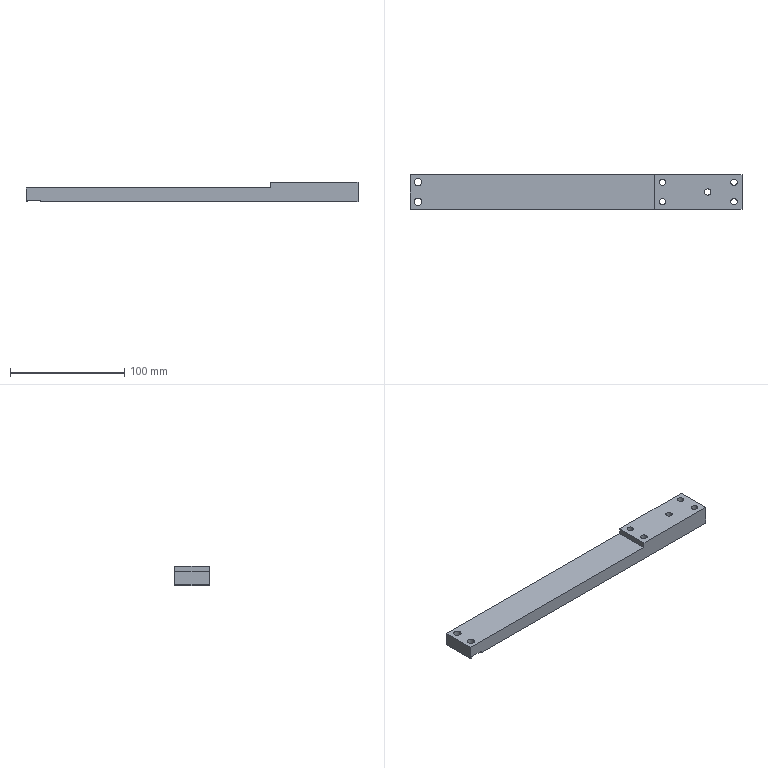Part | NX | features BREP 1 | 1 solid | 45 faces | box 290 x 30 x 17 mm | volume 111085 mm3 | cylinder 26 | plane 17 | cone 2 | commonest cylinder face diameters 5.5 x10 10 x10 6.5 x4 3.3 x2
STEP:
#1=CARTESIAN_POINT('',(-455.312,44.77,5.));
#2=VERTEX_POINT('',#1);
#3=CARTESIAN_POINT('',(-465.312,44.77,5.));
#4=VERTEX_POINT('',#3);
#5=CARTESIAN_POINT('',(-460.312,44.77,5.));
#6=DIRECTION('',(0.,0.,-1.));
#7=DIRECTION('',(-1.,0.,0.));
#8=AXIS2_PLACEMENT_3D('',#5,#6,#7);
#9=CIRCLE('',#8,5.);
#10=EDGE_CURVE('',#2,#4,#9,.T.);
#11=ORIENTED_EDGE('',*,*,#10,.F.);
#12=CARTESIAN_POINT('',(-455.312,44.77,0.));
#13=VERTEX_POINT('',#12);
#14=CARTESIAN_POINT('',(-455.312,44.77,0.));
#15=DIRECTION('',(0.,0.,-1.));
#16=VECTOR('',#15,1000.);
#17=LINE('',#14,#16);
#18=EDGE_CURVE('',#2,#13,#17,.T.);
#19=ORIENTED_EDGE('',*,*,#18,.T.);
#20=CARTESIAN_POINT('',(-465.312,44.77,0.));
#21=VERTEX_POINT('',#20);
#22=CARTESIAN_POINT('',(-460.312,44.77,0.));
#23=DIRECTION('',(0.,0.,-1.));
#24=DIRECTION('',(-1.,0.,0.));
#25=AXIS2_PLACEMENT_3D('',#22,#23,#24);
#26=CIRCLE('',#25,5.);
#27=EDGE_CURVE('',#13,#21,#26,.T.);
#28=ORIENTED_EDGE('',*,*,#27,.T.);
#29=CARTESIAN_POINT('',(-465.312,44.77,0.));
#30=DIRECTION('',(0.,0.,-1.));
#31=VECTOR('',#30,1000.);
#32=LINE('',#29,#31);
#33=EDGE_CURVE('',#4,#21,#32,.T.);
#34=ORIENTED_EDGE('',*,*,#33,.F.);
#35=EDGE_LOOP('',(#11,#19,#28,#34));
#36=FACE_BOUND('',#35,.T.);
#37=CARTESIAN_POINT('',(-460.312,44.77,0.));
#38=DIRECTION('',(0.,0.,-1.));
#39=DIRECTION('',(-1.,0.,0.));
#40=AXIS2_PLACEMENT_3D('',#37,#38,#39);
#41=CYLINDRICAL_SURFACE('',#40,5.);
#42=ADVANCED_FACE('',(#36),#41,.F.);
#43=CARTESIAN_POINT('',(-463.062,44.77,17.));
#44=VERTEX_POINT('',#43);
#45=CARTESIAN_POINT('',(-457.562,44.77,17.));
#46=VERTEX_POINT('',#45);
#47=CARTESIAN_POINT('',(-460.312,44.77,17.));
#48=DIRECTION('',(0.,0.,1.));
#49=DIRECTION('',(1.,0.,0.));
#50=AXIS2_PLACEMENT_3D('',#47,#48,#49);
#51=CIRCLE('',#50,2.75);
#52=EDGE_CURVE('',#44,#46,#51,.T.);
#53=ORIENTED_EDGE('',*,*,#52,.T.);
#54=CARTESIAN_POINT('',(-457.562,44.77,5.));
#55=VERTEX_POINT('',#54);
#56=CARTESIAN_POINT('',(-457.562,44.77,0.));
#57=DIRECTION('',(0.,0.,-1.));
#58=VECTOR('',#57,1000.);
#59=LINE('',#56,#58);
#60=EDGE_CURVE('',#46,#55,#59,.T.);
#61=ORIENTED_EDGE('',*,*,#60,.T.);
#62=CARTESIAN_POINT('',(-463.062,44.77,5.));
#63=VERTEX_POINT('',#62);
#64=CARTESIAN_POINT('',(-460.312,44.77,5.));
#65=DIRECTION('',(0.,0.,-1.));
#66=DIRECTION('',(-1.,0.,0.));
#67=AXIS2_PLACEMENT_3D('',#64,#65,#66);
#68=CIRCLE('',#67,2.75);
#69=EDGE_CURVE('',#55,#63,#68,.T.);
#70=ORIENTED_EDGE('',*,*,#69,.T.);
#71=CARTESIAN_POINT('',(-463.062,44.77,0.));
#72=DIRECTION('',(0.,0.,-1.));
#73=VECTOR('',#72,1000.);
#74=LINE('',#71,#73);
#75=EDGE_CURVE('',#44,#63,#74,.T.);
#76=ORIENTED_EDGE('',*,*,#75,.F.);
#77=EDGE_LOOP('',(#53,#61,#70,#76));
#78=FACE_BOUND('',#77,.T.);
#79=CARTESIAN_POINT('',(-460.312,44.77,0.));
#80=DIRECTION('',(0.,0.,-1.));
#81=DIRECTION('',(-1.,0.,0.));
#82=AXIS2_PLACEMENT_3D('',#79,#80,#81);
#83=CYLINDRICAL_SURFACE('',#82,2.75);
#84=ADVANCED_FACE('',(#78),#83,.F.);
#85=CARTESIAN_POINT('',(-455.312,27.77,5.));
#86=VERTEX_POINT('',#85);
#87=CARTESIAN_POINT('',(-465.312,27.77,5.));
#88=VERTEX_POINT('',#87);
#89=CARTESIAN_POINT('',(-460.312,27.77,5.));
#90=DIRECTION('',(0.,0.,-1.));
#91=DIRECTION('',(-1.,0.,0.));
#92=AXIS2_PLACEMENT_3D('',#89,#90,#91);
#93=CIRCLE('',#92,5.);
#94=EDGE_CURVE('',#86,#88,#93,.T.);
#95=ORIENTED_EDGE('',*,*,#94,.F.);
#96=CARTESIAN_POINT('',(-455.312,27.77,0.));
#97=VERTEX_POINT('',#96);
#98=CARTESIAN_POINT('',(-455.312,27.77,0.));
#99=DIRECTION('',(0.,0.,-1.));
#100=VECTOR('',#99,1000.);
#101=LINE('',#98,#100);
#102=EDGE_CURVE('',#86,#97,#101,.T.);
#103=ORIENTED_EDGE('',*,*,#102,.T.);
#104=CARTESIAN_POINT('',(-465.312,27.77,0.));
#105=VERTEX_POINT('',#104);
#106=CARTESIAN_POINT('',(-460.312,27.77,0.));
#107=DIRECTION('',(0.,0.,-1.));
#108=DIRECTION('',(-1.,0.,0.));
#109=AXIS2_PLACEMENT_3D('',#106,#107,#108);
#110=CIRCLE('',#109,5.);
#111=EDGE_CURVE('',#97,#105,#110,.T.);
#112=ORIENTED_EDGE('',*,*,#111,.T.);
#113=CARTESIAN_POINT('',(-465.312,27.77,0.));
#114=DIRECTION('',(0.,0.,-1.));
#115=VECTOR('',#114,1000.);
#116=LINE('',#113,#115);
#117=EDGE_CURVE('',#88,#105,#116,.T.);
#118=ORIENTED_EDGE('',*,*,#117,.F.);
#119=EDGE_LOOP('',(#95,#103,#112,#118));
#120=FACE_BOUND('',#119,.T.);
#121=CARTESIAN_POINT('',(-460.312,27.77,0.));
#122=DIRECTION('',(0.,0.,-1.));
#123=DIRECTION('',(-1.,0.,0.));
#124=AXIS2_PLACEMENT_3D('',#121,#122,#123);
#125=CYLINDRICAL_SURFACE('',#124,5.);
#126=ADVANCED_FACE('',(#120),#125,.F.);
#127=CARTESIAN_POINT('',(-463.062,27.77,17.));
#128=VERTEX_POINT('',#127);
#129=CARTESIAN_POINT('',(-457.562,27.77,17.));
#130=VERTEX_POINT('',#129);
#131=CARTESIAN_POINT('',(-460.312,27.77,17.));
#132=DIRECTION('',(0.,0.,1.));
#133=DIRECTION('',(1.,0.,0.));
#134=AXIS2_PLACEMENT_3D('',#131,#132,#133);
#135=CIRCLE('',#134,2.75);
#136=EDGE_CURVE('',#128,#130,#135,.T.);
#137=ORIENTED_EDGE('',*,*,#136,.T.);
#138=CARTESIAN_POINT('',(-457.562,27.77,5.));
#139=VERTEX_POINT('',#138);
#140=CARTESIAN_POINT('',(-457.562,27.77,0.));
#141=DIRECTION('',(0.,0.,-1.));
#142=VECTOR('',#141,1000.);
#143=LINE('',#140,#142);
#144=EDGE_CURVE('',#130,#139,#143,.T.);
#145=ORIENTED_EDGE('',*,*,#144,.T.);
#146=CARTESIAN_POINT('',(-463.062,27.77,5.));
#147=VERTEX_POINT('',#146);
#148=CARTESIAN_POINT('',(-460.312,27.77,5.));
#149=DIRECTION('',(0.,0.,-1.));
#150=DIRECTION('',(-1.,0.,0.));
#151=AXIS2_PLACEMENT_3D('',#148,#149,#150);
#152=CIRCLE('',#151,2.75);
#153=EDGE_CURVE('',#139,#147,#152,.T.);
#154=ORIENTED_EDGE('',*,*,#153,.T.);
#155=CARTESIAN_POINT('',(-463.062,27.77,0.));
#156=DIRECTION('',(0.,0.,-1.));
#157=VECTOR('',#156,1000.);
#158=LINE('',#155,#157);
#159=EDGE_CURVE('',#128,#147,#158,.T.);
#160=ORIENTED_EDGE('',*,*,#159,.F.);
#161=EDGE_LOOP('',(#137,#145,#154,#160));
#162=FACE_BOUND('',#161,.T.);
#163=CARTESIAN_POINT('',(-460.312,27.77,0.));
#164=DIRECTION('',(0.,0.,-1.));
#165=DIRECTION('',(-1.,0.,0.));
#166=AXIS2_PLACEMENT_3D('',#163,#164,#165);
#167=CYLINDRICAL_SURFACE('',#166,2.75);
#168=ADVANCED_FACE('',(#162),#167,.F.);
#169=CARTESIAN_POINT('',(-517.812,44.77,5.));
#170=VERTEX_POINT('',#169);
#171=CARTESIAN_POINT('',(-527.812,44.77,5.));
#172=VERTEX_POINT('',#171);
#173=CARTESIAN_POINT('',(-522.812,44.77,5.));
#174=DIRECTION('',(0.,0.,-1.));
#175=DIRECTION('',(-1.,0.,0.));
#176=AXIS2_PLACEMENT_3D('',#173,#174,#175);
#177=CIRCLE('',#176,5.);
#178=EDGE_CURVE('',#170,#172,#177,.T.);
#179=ORIENTED_EDGE('',*,*,#178,.F.);
#180=CARTESIAN_POINT('',(-517.812,44.77,0.));
#181=VERTEX_POINT('',#180);
#182=CARTESIAN_POINT('',(-517.812,44.77,0.));
#183=DIRECTION('',(0.,0.,-1.));
#184=VECTOR('',#183,1000.);
#185=LINE('',#182,#184);
#186=EDGE_CURVE('',#170,#181,#185,.T.);
#187=ORIENTED_EDGE('',*,*,#186,.T.);
#188=CARTESIAN_POINT('',(-527.812,44.77,0.));
#189=VERTEX_POINT('',#188);
#190=CARTESIAN_POINT('',(-522.812,44.77,0.));
#191=DIRECTION('',(0.,0.,-1.));
#192=DIRECTION('',(-1.,0.,0.));
#193=AXIS2_PLACEMENT_3D('',#190,#191,#192);
#194=CIRCLE('',#193,5.);
#195=EDGE_CURVE('',#181,#189,#194,.T.);
#196=ORIENTED_EDGE('',*,*,#195,.T.);
#197=CARTESIAN_POINT('',(-527.812,44.77,0.));
#198=DIRECTION('',(0.,0.,-1.));
#199=VECTOR('',#198,1000.);
#200=LINE('',#197,#199);
#201=EDGE_CURVE('',#172,#189,#200,.T.);
#202=ORIENTED_EDGE('',*,*,#201,.F.);
#203=EDGE_LOOP('',(#179,#187,#196,#202));
#204=FACE_BOUND('',#203,.T.);
#205=CARTESIAN_POINT('',(-522.812,44.77,0.));
#206=DIRECTION('',(0.,0.,-1.));
#207=DIRECTION('',(-1.,0.,0.));
#208=AXIS2_PLACEMENT_3D('',#205,#206,#207);
#209=CYLINDRICAL_SURFACE('',#208,5.);
#210=ADVANCED_FACE('',(#204),#209,.F.);
#211=CARTESIAN_POINT('',(-525.562,44.77,17.));
#212=VERTEX_POINT('',#211);
#213=CARTESIAN_POINT('',(-520.062,44.77,17.));
#214=VERTEX_POINT('',#213);
#215=CARTESIAN_POINT('',(-522.812,44.77,17.));
#216=DIRECTION('',(0.,0.,1.));
#217=DIRECTION('',(1.,0.,0.));
#218=AXIS2_PLACEMENT_3D('',#215,#216,#217);
#219=CIRCLE('',#218,2.75);
#220=EDGE_CURVE('',#212,#214,#219,.T.);
#221=ORIENTED_EDGE('',*,*,#220,.T.);
#222=CARTESIAN_POINT('',(-520.062,44.77,5.));
#223=VERTEX_POINT('',#222);
#224=CARTESIAN_POINT('',(-520.062,44.77,0.));
#225=DIRECTION('',(0.,0.,-1.));
#226=VECTOR('',#225,1000.);
#227=LINE('',#224,#226);
#228=EDGE_CURVE('',#214,#223,#227,.T.);
#229=ORIENTED_EDGE('',*,*,#228,.T.);
#230=CARTESIAN_POINT('',(-525.562,44.77,5.));
#231=VERTEX_POINT('',#230);
#232=CARTESIAN_POINT('',(-522.812,44.77,5.));
#233=DIRECTION('',(0.,0.,-1.));
#234=DIRECTION('',(-1.,0.,0.));
#235=AXIS2_PLACEMENT_3D('',#232,#233,#234);
#236=CIRCLE('',#235,2.75);
#237=EDGE_CURVE('',#223,#231,#236,.T.);
#238=ORIENTED_EDGE('',*,*,#237,.T.);
#239=CARTESIAN_POINT('',(-525.562,44.77,0.));
#240=DIRECTION('',(0.,0.,-1.));
#241=VECTOR('',#240,1000.);
#242=LINE('',#239,#241);
#243=EDGE_CURVE('',#212,#231,#242,.T.);
#244=ORIENTED_EDGE('',*,*,#243,.F.);
#245=EDGE_LOOP('',(#221,#229,#238,#244));
#246=FACE_BOUND('',#245,.T.);
#247=CARTESIAN_POINT('',(-522.812,44.77,0.));
#248=DIRECTION('',(0.,0.,-1.));
#249=DIRECTION('',(-1.,0.,0.));
#250=AXIS2_PLACEMENT_3D('',#247,#248,#249);
#251=CYLINDRICAL_SURFACE('',#250,2.75);
#252=ADVANCED_FACE('',(#246),#251,.F.);
#253=CARTESIAN_POINT('',(-517.812,27.77,5.));
#254=VERTEX_POINT('',#253);
#255=CARTESIAN_POINT('',(-527.812,27.77,5.));
#256=VERTEX_POINT('',#255);
#257=CARTESIAN_POINT('',(-522.812,27.77,5.));
#258=DIRECTION('',(0.,0.,-1.));
#259=DIRECTION('',(-1.,0.,0.));
#260=AXIS2_PLACEMENT_3D('',#257,#258,#259);
#261=CIRCLE('',#260,5.);
#262=EDGE_CURVE('',#254,#256,#261,.T.);
#263=ORIENTED_EDGE('',*,*,#262,.F.);
#264=CARTESIAN_POINT('',(-517.812,27.77,0.));
#265=VERTEX_POINT('',#264);
#266=CARTESIAN_POINT('',(-517.812,27.77,0.));
#267=DIRECTION('',(0.,0.,-1.));
#268=VECTOR('',#267,1000.);
#269=LINE('',#266,#268);
#270=EDGE_CURVE('',#254,#265,#269,.T.);
#271=ORIENTED_EDGE('',*,*,#270,.T.);
#272=CARTESIAN_POINT('',(-527.812,27.77,0.));
#273=VERTEX_POINT('',#272);
#274=CARTESIAN_POINT('',(-522.812,27.77,0.));
#275=DIRECTION('',(0.,0.,-1.));
#276=DIRECTION('',(-1.,0.,0.));
#277=AXIS2_PLACEMENT_3D('',#274,#275,#276);
#278=CIRCLE('',#277,5.);
#279=EDGE_CURVE('',#265,#273,#278,.T.);
#280=ORIENTED_EDGE('',*,*,#279,.T.);
#281=CARTESIAN_POINT('',(-527.812,27.77,0.));
#282=DIRECTION('',(0.,0.,-1.));
#283=VECTOR('',#282,1000.);
#284=LINE('',#281,#283);
#285=EDGE_CURVE('',#256,#273,#284,.T.);
#286=ORIENTED_EDGE('',*,*,#285,.F.);
#287=EDGE_LOOP('',(#263,#271,#280,#286));
#288=FACE_BOUND('',#287,.T.);
#289=CARTESIAN_POINT('',(-522.812,27.77,0.));
#290=DIRECTION('',(0.,0.,-1.));
#291=DIRECTION('',(-1.,0.,0.));
#292=AXIS2_PLACEMENT_3D('',#289,#290,#291);
#293=CYLINDRICAL_SURFACE('',#292,5.);
#294=ADVANCED_FACE('',(#288),#293,.F.);
#295=CARTESIAN_POINT('',(-525.562,27.77,17.));
#296=VERTEX_POINT('',#295);
#297=CARTESIAN_POINT('',(-520.062,27.77,17.));
#298=VERTEX_POINT('',#297);
#299=CARTESIAN_POINT('',(-522.812,27.77,17.));
#300=DIRECTION('',(0.,0.,1.));
#301=DIRECTION('',(1.,0.,0.));
#302=AXIS2_PLACEMENT_3D('',#299,#300,#301);
#303=CIRCLE('',#302,2.75);
#304=EDGE_CURVE('',#296,#298,#303,.T.);
#305=ORIENTED_EDGE('',*,*,#304,.T.);
#306=CARTESIAN_POINT('',(-520.062,27.77,5.));
#307=VERTEX_POINT('',#306);
#308=CARTESIAN_POINT('',(-520.062,27.77,0.));
#309=DIRECTION('',(0.,0.,-1.));
#310=VECTOR('',#309,1000.);
#311=LINE('',#308,#310);
#312=EDGE_CURVE('',#298,#307,#311,.T.);
#313=ORIENTED_EDGE('',*,*,#312,.T.);
#314=CARTESIAN_POINT('',(-525.562,27.77,5.));
#315=VERTEX_POINT('',#314);
#316=CARTESIAN_POINT('',(-522.812,27.77,5.));
#317=DIRECTION('',(0.,0.,-1.));
#318=DIRECTION('',(-1.,0.,0.));
#319=AXIS2_PLACEMENT_3D('',#316,#317,#318);
#320=CIRCLE('',#319,2.75);
#321=EDGE_CURVE('',#307,#315,#320,.T.);
#322=ORIENTED_EDGE('',*,*,#321,.T.);
#323=CARTESIAN_POINT('',(-525.562,27.77,0.));
#324=DIRECTION('',(0.,0.,-1.));
#325=VECTOR('',#324,1000.);
#326=LINE('',#323,#325);
#327=EDGE_CURVE('',#296,#315,#326,.T.);
#328=ORIENTED_EDGE('',*,*,#327,.F.);
#329=EDGE_LOOP('',(#305,#313,#322,#328));
#330=FACE_BOUND('',#329,.T.);
#331=CARTESIAN_POINT('',(-522.812,27.77,0.));
#332=DIRECTION('',(0.,0.,-1.));
#333=DIRECTION('',(-1.,0.,0.));
#334=AXIS2_PLACEMENT_3D('',#331,#332,#333);
#335=CYLINDRICAL_SURFACE('',#334,2.75);
#336=ADVANCED_FACE('',(#330),#335,.F.);
#337=CARTESIAN_POINT('',(-478.312,36.27,5.));
#338=VERTEX_POINT('',#337);
#339=CARTESIAN_POINT('',(-488.312,36.27,5.));
#340=VERTEX_POINT('',#339);
#341=CARTESIAN_POINT('',(-483.312,36.27,5.));
#342=DIRECTION('',(0.,0.,-1.));
#343=DIRECTION('',(-1.,0.,0.));
#344=AXIS2_PLACEMENT_3D('',#341,#342,#343);
#345=CIRCLE('',#344,5.);
#346=EDGE_CURVE('',#338,#340,#345,.T.);
#347=ORIENTED_EDGE('',*,*,#346,.F.);
#348=CARTESIAN_POINT('',(-478.312,36.27,0.));
#349=VERTEX_POINT('',#348);
#350=CARTESIAN_POINT('',(-478.312,36.27,0.));
#351=DIRECTION('',(0.,0.,-1.));
#352=VECTOR('',#351,1000.);
#353=LINE('',#350,#352);
#354=EDGE_CURVE('',#338,#349,#353,.T.);
#355=ORIENTED_EDGE('',*,*,#354,.T.);
#356=CARTESIAN_POINT('',(-488.312,36.27,0.));
#357=VERTEX_POINT('',#356);
#358=CARTESIAN_POINT('',(-483.312,36.27,0.));
#359=DIRECTION('',(0.,0.,-1.));
#360=DIRECTION('',(-1.,0.,0.));
#361=AXIS2_PLACEMENT_3D('',#358,#359,#360);
#362=CIRCLE('',#361,5.);
#363=EDGE_CURVE('',#349,#357,#362,.T.);
#364=ORIENTED_EDGE('',*,*,#363,.T.);
#365=CARTESIAN_POINT('',(-488.312,36.27,0.));
#366=DIRECTION('',(0.,0.,-1.));
#367=VECTOR('',#366,1000.);
#368=LINE('',#365,#367);
#369=EDGE_CURVE('',#340,#357,#368,.T.);
#370=ORIENTED_EDGE('',*,*,#369,.F.);
#371=EDGE_LOOP('',(#347,#355,#364,#370));
#372=FACE_BOUND('',#371,.T.);
#373=CARTESIAN_POINT('',(-483.312,36.27,0.));
#374=DIRECTION('',(0.,0.,-1.));
#375=DIRECTION('',(-1.,0.,0.));
#376=AXIS2_PLACEMENT_3D('',#373,#374,#375);
#377=CYLINDRICAL_SURFACE('',#376,5.);
#378=ADVANCED_FACE('',(#372),#377,.F.);
#379=CARTESIAN_POINT('',(-486.062,36.27,17.));
#380=VERTEX_POINT('',#379);
#381=CARTESIAN_POINT('',(-480.562,36.27,17.));
#382=VERTEX_POINT('',#381);
#383=CARTESIAN_POINT('',(-483.312,36.27,17.));
#384=DIRECTION('',(0.,0.,1.));
#385=DIRECTION('',(1.,0.,0.));
#386=AXIS2_PLACEMENT_3D('',#383,#384,#385);
#387=CIRCLE('',#386,2.75);
#388=EDGE_CURVE('',#380,#382,#387,.T.);
#389=ORIENTED_EDGE('',*,*,#388,.T.);
#390=CARTESIAN_POINT('',(-480.562,36.27,5.));
#391=VERTEX_POINT('',#390);
#392=CARTESIAN_POINT('',(-480.562,36.27,0.));
#393=DIRECTION('',(0.,0.,-1.));
#394=VECTOR('',#393,1000.);
#395=LINE('',#392,#394);
#396=EDGE_CURVE('',#382,#391,#395,.T.);
#397=ORIENTED_EDGE('',*,*,#396,.T.);
#398=CARTESIAN_POINT('',(-486.062,36.27,5.));
#399=VERTEX_POINT('',#398);
#400=CARTESIAN_POINT('',(-483.312,36.27,5.));
#401=DIRECTION('',(0.,0.,-1.));
#402=DIRECTION('',(-1.,0.,0.));
#403=AXIS2_PLACEMENT_3D('',#400,#401,#402);
#404=CIRCLE('',#403,2.75);
#405=EDGE_CURVE('',#391,#399,#404,.T.);
#406=ORIENTED_EDGE('',*,*,#405,.T.);
#407=CARTESIAN_POINT('',(-486.062,36.27,0.));
#408=DIRECTION('',(0.,0.,-1.));
#409=VECTOR('',#408,1000.);
#410=LINE('',#407,#409);
#411=EDGE_CURVE('',#380,#399,#410,.T.);
#412=ORIENTED_EDGE('',*,*,#411,.F.);
#413=EDGE_LOOP('',(#389,#397,#406,#412));
#414=FACE_BOUND('',#413,.T.);
#415=CARTESIAN_POINT('',(-483.312,36.27,0.));
#416=DIRECTION('',(0.,0.,-1.));
#417=DIRECTION('',(-1.,0.,0.));
#418=AXIS2_PLACEMENT_3D('',#415,#416,#417);
#419=CYLINDRICAL_SURFACE('',#418,2.75);
#420=ADVANCED_FACE('',(#414),#419,.F.);
#421=CARTESIAN_POINT('',(-739.562,27.77,1.5));
#422=VERTEX_POINT('',#421);
#423=CARTESIAN_POINT('',(-733.062,27.77,1.5));
#424=VERTEX_POINT('',#423);
#425=CARTESIAN_POINT('',(-736.312,27.77,1.5));
#426=DIRECTION('',(0.,0.,1.));
#427=DIRECTION('',(1.,0.,0.));
#428=AXIS2_PLACEMENT_3D('',#425,#426,#427);
#429=CIRCLE('',#428,3.25);
#430=EDGE_CURVE('',#422,#424,#429,.T.);
#431=ORIENTED_EDGE('',*,*,#430,.F.);
#432=CARTESIAN_POINT('',(-739.562,27.77,12.));
#433=VERTEX_POINT('',#432);
#434=CARTESIAN_POINT('',(-739.562,27.77,0.));
#435=DIRECTION('',(0.,0.,1.));
#436=VECTOR('',#435,1000.);
#437=LINE('',#434,#436);
#438=EDGE_CURVE('',#433,#422,#437,.F.);
#439=ORIENTED_EDGE('',*,*,#438,.F.);
#440=CARTESIAN_POINT('',(-733.062,27.77,12.));
#441=VERTEX_POINT('',#440);
#442=CARTESIAN_POINT('',(-736.312,27.77,12.));
#443=DIRECTION('',(0.,0.,1.));
#444=DIRECTION('',(1.,0.,0.));
#445=AXIS2_PLACEMENT_3D('',#442,#443,#444);
#446=CIRCLE('',#445,3.25);
#447=EDGE_CURVE('',#433,#441,#446,.T.);
#448=ORIENTED_EDGE('',*,*,#447,.T.);
#449=CARTESIAN_POINT('',(-733.062,27.77,0.));
#450=DIRECTION('',(0.,0.,1.));
#451=VECTOR('',#450,1000.);
#452=LINE('',#449,#451);
#453=EDGE_CURVE('',#441,#424,#452,.F.);
#454=ORIENTED_EDGE('',*,*,#453,.T.);
#455=EDGE_LOOP('',(#431,#439,#448,#454));
#456=FACE_BOUND('',#455,.T.);
#457=CARTESIAN_POINT('',(-736.312,27.77,0.));
#458=DIRECTION('',(0.,0.,1.));
#459=DIRECTION('',(1.,0.,0.));
#460=AXIS2_PLACEMENT_3D('',#457,#458,#459);
#461=CYLINDRICAL_SURFACE('',#460,3.25);
#462=ADVANCED_FACE('',(#456),#461,.F.);
#463=CARTESIAN_POINT('',(-739.562,44.77,1.5));
#464=VERTEX_POINT('',#463);
#465=CARTESIAN_POINT('',(-733.062,44.77,1.5));
#466=VERTEX_POINT('',#465);
#467=CARTESIAN_POINT('',(-736.312,44.77,1.5));
#468=DIRECTION('',(0.,0.,1.));
#469=DIRECTION('',(1.,0.,0.));
#470=AXIS2_PLACEMENT_3D('',#467,#468,#469);
#471=CIRCLE('',#470,3.25);
#472=EDGE_CURVE('',#464,#466,#471,.T.);
#473=ORIENTED_EDGE('',*,*,#472,.F.);
#474=CARTESIAN_POINT('',(-739.562,44.77,12.));
#475=VERTEX_POINT('',#474);
#476=CARTESIAN_POINT('',(-739.562,44.77,0.));
#477=DIRECTION('',(0.,0.,1.));
#478=VECTOR('',#477,1000.);
#479=LINE('',#476,#478);
#480=EDGE_CURVE('',#475,#464,#479,.F.);
#481=ORIENTED_EDGE('',*,*,#480,.F.);
#482=CARTESIAN_POINT('',(-733.062,44.77,12.));
#483=VERTEX_POINT('',#482);
#484=CARTESIAN_POINT('',(-736.312,44.77,12.));
#485=DIRECTION('',(0.,0.,1.));
#486=DIRECTION('',(1.,0.,0.));
#487=AXIS2_PLACEMENT_3D('',#484,#485,#486);
#488=CIRCLE('',#487,3.25);
#489=EDGE_CURVE('',#475,#483,#488,.T.);
#490=ORIENTED_EDGE('',*,*,#489,.T.);
#491=CARTESIAN_POINT('',(-733.062,44.77,0.));
#492=DIRECTION('',(0.,0.,1.));
#493=VECTOR('',#492,1000.);
#494=LINE('',#491,#493);
#495=EDGE_CURVE('',#483,#466,#494,.F.);
#496=ORIENTED_EDGE('',*,*,#495,.T.);
#497=EDGE_LOOP('',(#473,#481,#490,#496));
#498=FACE_BOUND('',#497,.T.);
#499=CARTESIAN_POINT('',(-736.312,44.77,0.));
#500=DIRECTION('',(0.,0.,1.));
#501=DIRECTION('',(1.,0.,0.));
#502=AXIS2_PLACEMENT_3D('',#499,#500,#501);
#503=CYLINDRICAL_SURFACE('',#502,3.25);
#504=ADVANCED_FACE('',(#498),#503,.F.);
#505=CARTESIAN_POINT('',(-684.662,36.27,10.1));
#506=VERTEX_POINT('',#505);
#507=CARTESIAN_POINT('',(-687.962,36.27,10.1));
#508=VERTEX_POINT('',#507);
#509=CARTESIAN_POINT('',(-686.312,36.27,10.1));
#510=DIRECTION('',(0.,0.,-1.));
#511=DIRECTION('',(-1.,0.,0.));
#512=AXIS2_PLACEMENT_3D('',#509,#510,#511);
#513=CIRCLE('',#512,1.65);
#514=EDGE_CURVE('',#506,#508,#513,.T.);
#515=ORIENTED_EDGE('',*,*,#514,.F.);
#516=CARTESIAN_POINT('',(-684.662,36.27,0.));
#517=VERTEX_POINT('',#516);
#518=CARTESIAN_POINT('',(-684.662,36.27,0.));
#519=DIRECTION('',(0.,0.,-1.));
#520=VECTOR('',#519,1000.);
#521=LINE('',#518,#520);
#522=EDGE_CURVE('',#506,#517,#521,.T.);
#523=ORIENTED_EDGE('',*,*,#522,.T.);
#524=CARTESIAN_POINT('',(-687.962,36.27,0.));
#525=VERTEX_POINT('',#524);
#526=CARTESIAN_POINT('',(-686.312,36.27,0.));
#527=DIRECTION('',(0.,0.,-1.));
#528=DIRECTION('',(-1.,0.,0.));
#529=AXIS2_PLACEMENT_3D('',#526,#527,#528);
#530=CIRCLE('',#529,1.65);
#531=EDGE_CURVE('',#517,#525,#530,.T.);
#532=ORIENTED_EDGE('',*,*,#531,.T.);
#533=CARTESIAN_POINT('',(-687.962,36.27,0.));
#534=DIRECTION('',(0.,0.,-1.));
#535=VECTOR('',#534,1000.);
#536=LINE('',#533,#535);
#537=EDGE_CURVE('',#508,#525,#536,.T.);
#538=ORIENTED_EDGE('',*,*,#537,.F.);
#539=EDGE_LOOP('',(#515,#523,#532,#538));
#540=FACE_BOUND('',#539,.T.);
#541=CARTESIAN_POINT('',(-686.312,36.27,0.));
#542=DIRECTION('',(0.,0.,-1.));
#543=DIRECTION('',(-1.,0.,0.));
#544=AXIS2_PLACEMENT_3D('',#541,#542,#543);
#545=CYLINDRICAL_SURFACE('',#544,1.65);
#546=ADVANCED_FACE('',(#540),#545,.F.);
#547=CARTESIAN_POINT('',(-686.312,36.27,11.091));
#548=VERTEX_POINT('',#547);
#549=CARTESIAN_POINT('',(-687.962,36.27,10.1));
#550=DIRECTION('',(-0.8572,0.,-0.515));
#551=VECTOR('',#550,1000.);
#552=LINE('',#549,#551);
#553=EDGE_CURVE('',#548,#508,#552,.T.);
#554=ORIENTED_EDGE('',*,*,#553,.F.);
#555=CARTESIAN_POINT('',(-684.662,36.27,10.1));
#556=DIRECTION('',(0.8572,0.,-0.515));
#557=VECTOR('',#556,1000.);
#558=LINE('',#555,#557);
#559=EDGE_CURVE('',#548,#506,#558,.T.);
#560=ORIENTED_EDGE('',*,*,#559,.T.);
#561=ORIENTED_EDGE('',*,*,#514,.T.);
#562=EDGE_LOOP('',(#554,#560,#561));
#563=FACE_BOUND('',#562,.T.);
#564=CARTESIAN_POINT('',(-686.312,36.27,10.1));
#565=DIRECTION('',(0.,0.,-1.));
#566=DIRECTION('',(-1.,0.,0.));
#567=AXIS2_PLACEMENT_3D('',#564,#565,#566);
#568=CONICAL_SURFACE('',#567,1.65,1.03);
#569=ADVANCED_FACE('',(#563),#568,.F.);
#570=CARTESIAN_POINT('',(-742.312,21.27,0.));
#571=VERTEX_POINT('',#570);
#572=CARTESIAN_POINT('',(-742.312,51.27,0.));
#573=VERTEX_POINT('',#572);
#574=CARTESIAN_POINT('',(-742.312,51.27,0.));
#575=DIRECTION('',(0.,1.,0.));
#576=VECTOR('',#575,1000.);
#577=LINE('',#574,#576);
#578=EDGE_CURVE('',#571,#573,#577,.T.);
#579=ORIENTED_EDGE('',*,*,#578,.F.);
#580=CARTESIAN_POINT('',(-743.312,21.27,0.));
#581=VERTEX_POINT('',#580);
#582=CARTESIAN_POINT('',(-743.312,21.27,0.));
#583=DIRECTION('',(1.,0.,0.));
#584=VECTOR('',#583,1000.);
#585=LINE('',#582,#584);
#586=EDGE_CURVE('',#581,#571,#585,.T.);
#587=ORIENTED_EDGE('',*,*,#586,.F.);
#588=CARTESIAN_POINT('',(-743.312,51.27,0.));
#589=VERTEX_POINT('',#588);
#590=CARTESIAN_POINT('',(-743.312,21.27,0.));
#591=DIRECTION('',(0.,-1.,0.));
#592=VECTOR('',#591,1000.);
#593=LINE('',#590,#592);
#594=EDGE_CURVE('',#589,#581,#593,.T.);
#595=ORIENTED_EDGE('',*,*,#594,.F.);
#596=CARTESIAN_POINT('',(-743.312,51.27,0.));
#597=DIRECTION('',(-1.,0.,0.));
#598=VECTOR('',#597,1000.);
#599=LINE('',#596,#598);
#600=EDGE_CURVE('',#573,#589,#599,.T.);
#601=ORIENTED_EDGE('',*,*,#600,.F.);
#602=EDGE_LOOP('',(#579,#587,#595,#601));
#603=FACE_BOUND('',#602,.T.);
#604=CARTESIAN_POINT('',(-743.312,51.27,0.));
#605=DIRECTION('',(0.,0.,-1.));
#606=DIRECTION('',(0.,-1.,0.));
#607=AXIS2_PLACEMENT_3D('',#604,#605,#606);
#608=PLANE('',#607);
#609=ADVANCED_FACE('',(#603),#608,.T.);
#610=ORIENTED_EDGE('',*,*,#594,.T.);
#611=CARTESIAN_POINT('',(-743.312,21.27,12.));
#612=VERTEX_POINT('',#611);
#613=CARTESIAN_POINT('',(-743.312,21.27,12.));
#614=DIRECTION('',(0.,0.,-1.));
#615=VECTOR('',#614,1000.);
#616=LINE('',#613,#615);
#617=EDGE_CURVE('',#612,#581,#616,.T.);
#618=ORIENTED_EDGE('',*,*,#617,.F.);
#619=CARTESIAN_POINT('',(-743.312,51.27,12.));
#620=VERTEX_POINT('',#619);
#621=CARTESIAN_POINT('',(-743.312,21.27,12.));
#622=DIRECTION('',(0.,-1.,0.));
#623=VECTOR('',#622,1000.);
#624=LINE('',#621,#623);
#625=EDGE_CURVE('',#620,#612,#624,.T.);
#626=ORIENTED_EDGE('',*,*,#625,.F.);
#627=CARTESIAN_POINT('',(-743.312,51.27,12.));
#628=DIRECTION('',(0.,0.,-1.));
#629=VECTOR('',#628,1000.);
#630=LINE('',#627,#629);
#631=EDGE_CURVE('',#620,#589,#630,.T.);
#632=ORIENTED_EDGE('',*,*,#631,.T.);
#633=EDGE_LOOP('',(#610,#618,#626,#632));
#634=FACE_BOUND('',#633,.T.);
#635=CARTESIAN_POINT('',(-743.312,21.27,12.));
#636=DIRECTION('',(1.,0.,0.));
#637=DIRECTION('',(0.,1.,0.));
#638=AXIS2_PLACEMENT_3D('',#635,#636,#637);
#639=PLANE('',#638);
#640=ADVANCED_FACE('',(#634),#639,.F.);
#641=ORIENTED_EDGE('',*,*,#586,.T.);
#642=CARTESIAN_POINT('',(-742.312,21.27,1.5));
#643=VERTEX_POINT('',#642);
#644=CARTESIAN_POINT('',(-742.312,21.27,12.));
#645=DIRECTION('',(0.,0.,1.));
#646=VECTOR('',#645,1000.);
#647=LINE('',#644,#646);
#648=EDGE_CURVE('',#571,#643,#647,.T.);
#649=ORIENTED_EDGE('',*,*,#648,.T.);
#650=CARTESIAN_POINT('',(-730.312,21.27,1.5));
#651=VERTEX_POINT('',#650);
#652=CARTESIAN_POINT('',(-743.312,21.27,1.5));
#653=DIRECTION('',(1.,0.,0.));
#654=VECTOR('',#653,1000.);
#655=LINE('',#652,#654);
#656=EDGE_CURVE('',#643,#651,#655,.T.);
#657=ORIENTED_EDGE('',*,*,#656,.T.);
#658=CARTESIAN_POINT('',(-730.312,21.27,0.));
#659=VERTEX_POINT('',#658);
#660=CARTESIAN_POINT('',(-730.312,21.27,12.));
#661=DIRECTION('',(0.,0.,-1.));
#662=VECTOR('',#661,1000.);
#663=LINE('',#660,#662);
#664=EDGE_CURVE('',#651,#659,#663,.T.);
#665=ORIENTED_EDGE('',*,*,#664,.T.);
#666=CARTESIAN_POINT('',(-453.312,21.27,0.));
#667=VERTEX_POINT('',#666);
#668=CARTESIAN_POINT('',(-743.312,21.27,0.));
#669=DIRECTION('',(1.,0.,0.));
#670=VECTOR('',#669,1000.);
#671=LINE('',#668,#670);
#672=EDGE_CURVE('',#659,#667,#671,.T.);
#673=ORIENTED_EDGE('',*,*,#672,.T.);
#674=CARTESIAN_POINT('',(-453.312,21.27,17.));
#675=VERTEX_POINT('',#674);
#676=CARTESIAN_POINT('',(-453.312,21.27,12.));
#677=DIRECTION('',(0.,0.,-1.));
#678=VECTOR('',#677,1000.);
#679=LINE('',#676,#678);
#680=EDGE_CURVE('',#675,#667,#679,.T.);
#681=ORIENTED_EDGE('',*,*,#680,.F.);
#682=CARTESIAN_POINT('',(-529.312,21.27,17.));
#683=VERTEX_POINT('',#682);
#684=CARTESIAN_POINT('',(-453.312,21.27,17.));
#685=DIRECTION('',(-1.,0.,0.));
#686=VECTOR('',#685,1000.);
#687=LINE('',#684,#686);
#688=EDGE_CURVE('',#675,#683,#687,.T.);
#689=ORIENTED_EDGE('',*,*,#688,.T.);
#690=CARTESIAN_POINT('',(-529.312,21.27,12.));
#691=VERTEX_POINT('',#690);
#692=CARTESIAN_POINT('',(-529.312,21.27,12.));
#693=DIRECTION('',(0.,0.,-1.));
#694=VECTOR('',#693,1000.);
#695=LINE('',#692,#694);
#696=EDGE_CURVE('',#683,#691,#695,.T.);
#697=ORIENTED_EDGE('',*,*,#696,.T.);
#698=CARTESIAN_POINT('',(-743.312,21.27,12.));
#699=DIRECTION('',(1.,0.,0.));
#700=VECTOR('',#699,1000.);
#701=LINE('',#698,#700);
#702=EDGE_CURVE('',#612,#691,#701,.T.);
#703=ORIENTED_EDGE('',*,*,#702,.F.);
#704=ORIENTED_EDGE('',*,*,#617,.T.);
#705=EDGE_LOOP('',(#641,#649,#657,#665,#673,#681,#689,#697,#703,#704));
#706=FACE_BOUND('',#705,.T.);
#707=CARTESIAN_POINT('',(-743.312,21.27,12.));
#708=DIRECTION('',(0.,1.,0.));
#709=DIRECTION('',(1.,0.,0.));
#710=AXIS2_PLACEMENT_3D('',#707,#708,#709);
#711=PLANE('',#710);
#712=ADVANCED_FACE('',(#706),#711,.F.);
#713=CARTESIAN_POINT('',(-453.312,51.27,0.));
#714=VERTEX_POINT('',#713);
#715=CARTESIAN_POINT('',(-453.312,21.27,0.));
#716=DIRECTION('',(0.,1.,0.));
#717=VECTOR('',#716,1000.);
#718=LINE('',#715,#717);
#719=EDGE_CURVE('',#667,#714,#718,.T.);
#720=ORIENTED_EDGE('',*,*,#719,.T.);
#721=CARTESIAN_POINT('',(-453.312,51.27,17.));
#722=VERTEX_POINT('',#721);
#723=CARTESIAN_POINT('',(-453.312,51.27,12.));
#724=DIRECTION('',(0.,0.,-1.));
#725=VECTOR('',#724,1000.);
#726=LINE('',#723,#725);
#727=EDGE_CURVE('',#722,#714,#726,.T.);
#728=ORIENTED_EDGE('',*,*,#727,.F.);
#729=CARTESIAN_POINT('',(-453.312,-54.894,17.));
#730=DIRECTION('',(0.,1.,0.));
#731=VECTOR('',#730,1000.);
#732=LINE('',#729,#731);
#733=EDGE_CURVE('',#675,#722,#732,.T.);
#734=ORIENTED_EDGE('',*,*,#733,.F.);
#735=ORIENTED_EDGE('',*,*,#680,.T.);
#736=EDGE_LOOP('',(#720,#728,#734,#735));
#737=FACE_BOUND('',#736,.T.);
#738=CARTESIAN_POINT('',(-453.312,21.27,12.));
#739=DIRECTION('',(-1.,0.,0.));
#740=DIRECTION('',(0.,0.,1.));
#741=AXIS2_PLACEMENT_3D('',#738,#739,#740);
#742=PLANE('',#741);
#743=ADVANCED_FACE('',(#737),#742,.F.);
#744=CARTESIAN_POINT('',(-742.312,51.27,1.5));
#745=VERTEX_POINT('',#744);
#746=CARTESIAN_POINT('',(-730.312,51.27,1.5));
#747=VERTEX_POINT('',#746);
#748=CARTESIAN_POINT('',(-742.312,51.27,1.5));
#749=DIRECTION('',(1.,0.,0.));
#750=VECTOR('',#749,1000.);
#751=LINE('',#748,#750);
#752=EDGE_CURVE('',#745,#747,#751,.T.);
#753=ORIENTED_EDGE('',*,*,#752,.F.);
#754=CARTESIAN_POINT('',(-742.312,51.27,0.));
#755=DIRECTION('',(0.,0.,1.));
#756=VECTOR('',#755,1000.);
#757=LINE('',#754,#756);
#758=EDGE_CURVE('',#573,#745,#757,.T.);
#759=ORIENTED_EDGE('',*,*,#758,.F.);
#760=ORIENTED_EDGE('',*,*,#600,.T.);
#761=ORIENTED_EDGE('',*,*,#631,.F.);
#762=CARTESIAN_POINT('',(-529.312,51.27,12.));
#763=VERTEX_POINT('',#762);
#764=CARTESIAN_POINT('',(-743.312,51.27,12.));
#765=DIRECTION('',(-1.,0.,0.));
#766=VECTOR('',#765,1000.);
#767=LINE('',#764,#766);
#768=EDGE_CURVE('',#763,#620,#767,.T.);
#769=ORIENTED_EDGE('',*,*,#768,.F.);
#770=CARTESIAN_POINT('',(-529.312,51.27,17.));
#771=VERTEX_POINT('',#770);
#772=CARTESIAN_POINT('',(-529.312,51.27,12.));
#773=DIRECTION('',(0.,0.,1.));
#774=VECTOR('',#773,1000.);
#775=LINE('',#772,#774);
#776=EDGE_CURVE('',#763,#771,#775,.T.);
#777=ORIENTED_EDGE('',*,*,#776,.T.);
#778=CARTESIAN_POINT('',(-453.312,51.27,17.));
#779=DIRECTION('',(1.,0.,0.));
#780=VECTOR('',#779,1000.);
#781=LINE('',#778,#780);
#782=EDGE_CURVE('',#771,#722,#781,.T.);
#783=ORIENTED_EDGE('',*,*,#782,.T.);
#784=ORIENTED_EDGE('',*,*,#727,.T.);
#785=CARTESIAN_POINT('',(-730.312,51.27,0.));
#786=VERTEX_POINT('',#785);
#787=CARTESIAN_POINT('',(-743.312,51.27,0.));
#788=DIRECTION('',(-1.,0.,0.));
#789=VECTOR('',#788,1000.);
#790=LINE('',#787,#789);
#791=EDGE_CURVE('',#714,#786,#790,.T.);
#792=ORIENTED_EDGE('',*,*,#791,.T.);
#793=CARTESIAN_POINT('',(-730.312,51.27,0.));
#794=DIRECTION('',(0.,0.,-1.));
#795=VECTOR('',#794,1000.);
#796=LINE('',#793,#795);
#797=EDGE_CURVE('',#747,#786,#796,.T.);
#798=ORIENTED_EDGE('',*,*,#797,.F.);
#799=EDGE_LOOP('',(#753,#759,#760,#761,#769,#777,#783,#784,#792,#798));
#800=FACE_BOUND('',#799,.T.);
#801=CARTESIAN_POINT('',(-743.312,51.27,12.));
#802=DIRECTION('',(0.,-1.,0.));
#803=DIRECTION('',(0.,0.,-1.));
#804=AXIS2_PLACEMENT_3D('',#801,#802,#803);
#805=PLANE('',#804);
#806=ADVANCED_FACE('',(#800),#805,.F.);
#807=ORIENTED_EDGE('',*,*,#702,.T.);
#808=CARTESIAN_POINT('',(-529.312,-54.894,12.));
#809=DIRECTION('',(0.,1.,0.));
#810=VECTOR('',#809,1000.);
#811=LINE('',#808,#810);
#812=EDGE_CURVE('',#691,#763,#811,.T.);
#813=ORIENTED_EDGE('',*,*,#812,.T.);
#814=ORIENTED_EDGE('',*,*,#768,.T.);
#815=ORIENTED_EDGE('',*,*,#625,.T.);
#816=EDGE_LOOP('',(#807,#813,#814,#815));
#817=FACE_BOUND('',#816,.T.);
#818=CARTESIAN_POINT('',(-736.312,27.77,12.));
#819=DIRECTION('',(0.,0.,1.));
#820=DIRECTION('',(1.,0.,0.));
#821=AXIS2_PLACEMENT_3D('',#818,#819,#820);
#822=CIRCLE('',#821,3.25);
#823=EDGE_CURVE('',#441,#433,#822,.T.);
#824=ORIENTED_EDGE('',*,*,#823,.F.);
#825=ORIENTED_EDGE('',*,*,#447,.F.);
#826=EDGE_LOOP('',(#824,#825));
#827=FACE_BOUND('',#826,.T.);
#828=CARTESIAN_POINT('',(-736.312,44.77,12.));
#829=DIRECTION('',(0.,0.,1.));
#830=DIRECTION('',(1.,0.,0.));
#831=AXIS2_PLACEMENT_3D('',#828,#829,#830);
#832=CIRCLE('',#831,3.25);
#833=EDGE_CURVE('',#483,#475,#832,.T.);
#834=ORIENTED_EDGE('',*,*,#833,.F.);
#835=ORIENTED_EDGE('',*,*,#489,.F.);
#836=EDGE_LOOP('',(#834,#835));
#837=FACE_BOUND('',#836,.T.);
#838=CARTESIAN_POINT('',(-743.312,51.27,12.));
#839=DIRECTION('',(0.,0.,-1.));
#840=DIRECTION('',(0.,-1.,0.));
#841=AXIS2_PLACEMENT_3D('',#838,#839,#840);
#842=PLANE('',#841);
#843=ADVANCED_FACE('',(#817,#827,#837),#842,.F.);
#844=CARTESIAN_POINT('',(-730.312,51.27,0.));
#845=DIRECTION('',(0.,-1.,0.));
#846=VECTOR('',#845,1000.);
#847=LINE('',#844,#846);
#848=EDGE_CURVE('',#786,#659,#847,.T.);
#849=ORIENTED_EDGE('',*,*,#848,.F.);
#850=ORIENTED_EDGE('',*,*,#791,.F.);
#851=ORIENTED_EDGE('',*,*,#719,.F.);
#852=ORIENTED_EDGE('',*,*,#672,.F.);
#853=EDGE_LOOP('',(#849,#850,#851,#852));
#854=FACE_BOUND('',#853,.T.);
#855=CARTESIAN_POINT('',(-460.312,44.77,0.));
#856=DIRECTION('',(0.,0.,-1.));
#857=DIRECTION('',(-1.,0.,0.));
#858=AXIS2_PLACEMENT_3D('',#855,#856,#857);
#859=CIRCLE('',#858,5.);
#860=EDGE_CURVE('',#21,#13,#859,.T.);
#861=ORIENTED_EDGE('',*,*,#860,.F.);
#862=ORIENTED_EDGE('',*,*,#27,.F.);
#863=EDGE_LOOP('',(#861,#862));
#864=FACE_BOUND('',#863,.T.);
#865=CARTESIAN_POINT('',(-460.312,27.77,0.));
#866=DIRECTION('',(0.,0.,-1.));
#867=DIRECTION('',(-1.,0.,0.));
#868=AXIS2_PLACEMENT_3D('',#865,#866,#867);
#869=CIRCLE('',#868,5.);
#870=EDGE_CURVE('',#105,#97,#869,.T.);
#871=ORIENTED_EDGE('',*,*,#870,.F.);
#872=ORIENTED_EDGE('',*,*,#111,.F.);
#873=EDGE_LOOP('',(#871,#872));
#874=FACE_BOUND('',#873,.T.);
#875=CARTESIAN_POINT('',(-522.812,44.77,0.));
#876=DIRECTION('',(0.,0.,-1.));
#877=DIRECTION('',(-1.,0.,0.));
#878=AXIS2_PLACEMENT_3D('',#875,#876,#877);
#879=CIRCLE('',#878,5.);
#880=EDGE_CURVE('',#189,#181,#879,.T.);
#881=ORIENTED_EDGE('',*,*,#880,.F.);
#882=ORIENTED_EDGE('',*,*,#195,.F.);
#883=EDGE_LOOP('',(#881,#882));
#884=FACE_BOUND('',#883,.T.);
#885=CARTESIAN_POINT('',(-522.812,27.77,0.));
#886=DIRECTION('',(0.,0.,-1.));
#887=DIRECTION('',(-1.,0.,0.));
#888=AXIS2_PLACEMENT_3D('',#885,#886,#887);
#889=CIRCLE('',#888,5.);
#890=EDGE_CURVE('',#273,#265,#889,.T.);
#891=ORIENTED_EDGE('',*,*,#890,.F.);
#892=ORIENTED_EDGE('',*,*,#279,.F.);
#893=EDGE_LOOP('',(#891,#892));
#894=FACE_BOUND('',#893,.T.);
#895=CARTESIAN_POINT('',(-483.312,36.27,0.));
#896=DIRECTION('',(0.,0.,-1.));
#897=DIRECTION('',(-1.,0.,0.));
#898=AXIS2_PLACEMENT_3D('',#895,#896,#897);
#899=CIRCLE('',#898,5.);
#900=EDGE_CURVE('',#357,#349,#899,.T.);
#901=ORIENTED_EDGE('',*,*,#900,.F.);
#902=ORIENTED_EDGE('',*,*,#363,.F.);
#903=EDGE_LOOP('',(#901,#902));
#904=FACE_BOUND('',#903,.T.);
#905=CARTESIAN_POINT('',(-686.312,36.27,0.));
#906=DIRECTION('',(0.,0.,-1.));
#907=DIRECTION('',(-1.,0.,0.));
#908=AXIS2_PLACEMENT_3D('',#905,#906,#907);
#909=CIRCLE('',#908,1.65);
#910=EDGE_CURVE('',#525,#517,#909,.T.);
#911=ORIENTED_EDGE('',*,*,#910,.F.);
#912=ORIENTED_EDGE('',*,*,#531,.F.);
#913=EDGE_LOOP('',(#911,#912));
#914=FACE_BOUND('',#913,.T.);
#915=CARTESIAN_POINT('',(-743.312,51.27,0.));
#916=DIRECTION('',(0.,0.,-1.));
#917=DIRECTION('',(0.,-1.,0.));
#918=AXIS2_PLACEMENT_3D('',#915,#916,#917);
#919=PLANE('',#918);
#920=ADVANCED_FACE('',(#854,#864,#874,#884,#894,#904,#914),#919,.T.);
#921=ORIENTED_EDGE('',*,*,#688,.F.);
#922=ORIENTED_EDGE('',*,*,#733,.T.);
#923=ORIENTED_EDGE('',*,*,#782,.F.);
#924=CARTESIAN_POINT('',(-529.312,-54.894,17.));
#925=DIRECTION('',(0.,1.,0.));
#926=VECTOR('',#925,1000.);
#927=LINE('',#924,#926);
#928=EDGE_CURVE('',#683,#771,#927,.T.);
#929=ORIENTED_EDGE('',*,*,#928,.F.);
#930=EDGE_LOOP('',(#921,#922,#923,#929));
#931=FACE_BOUND('',#930,.T.);
#932=ORIENTED_EDGE('',*,*,#52,.F.);
#933=CARTESIAN_POINT('',(-460.312,44.77,17.));
#934=DIRECTION('',(0.,0.,1.));
#935=DIRECTION('',(1.,0.,0.));
#936=AXIS2_PLACEMENT_3D('',#933,#934,#935);
#937=CIRCLE('',#936,2.75);
#938=EDGE_CURVE('',#46,#44,#937,.T.);
#939=ORIENTED_EDGE('',*,*,#938,.F.);
#940=EDGE_LOOP('',(#932,#939));
#941=FACE_BOUND('',#940,.T.);
#942=ORIENTED_EDGE('',*,*,#136,.F.);
#943=CARTESIAN_POINT('',(-460.312,27.77,17.));
#944=DIRECTION('',(0.,0.,1.));
#945=DIRECTION('',(1.,0.,0.));
#946=AXIS2_PLACEMENT_3D('',#943,#944,#945);
#947=CIRCLE('',#946,2.75);
#948=EDGE_CURVE('',#130,#128,#947,.T.);
#949=ORIENTED_EDGE('',*,*,#948,.F.);
#950=EDGE_LOOP('',(#942,#949));
#951=FACE_BOUND('',#950,.T.);
#952=ORIENTED_EDGE('',*,*,#220,.F.);
#953=CARTESIAN_POINT('',(-522.812,44.77,17.));
#954=DIRECTION('',(0.,0.,1.));
#955=DIRECTION('',(1.,0.,0.));
#956=AXIS2_PLACEMENT_3D('',#953,#954,#955);
#957=CIRCLE('',#956,2.75);
#958=EDGE_CURVE('',#214,#212,#957,.T.);
#959=ORIENTED_EDGE('',*,*,#958,.F.);
#960=EDGE_LOOP('',(#952,#959));
#961=FACE_BOUND('',#960,.T.);
#962=ORIENTED_EDGE('',*,*,#304,.F.);
#963=CARTESIAN_POINT('',(-522.812,27.77,17.));
#964=DIRECTION('',(0.,0.,1.));
#965=DIRECTION('',(1.,0.,0.));
#966=AXIS2_PLACEMENT_3D('',#963,#964,#965);
#967=CIRCLE('',#966,2.75);
#968=EDGE_CURVE('',#298,#296,#967,.T.);
#969=ORIENTED_EDGE('',*,*,#968,.F.);
#970=EDGE_LOOP('',(#962,#969));
#971=FACE_BOUND('',#970,.T.);
#972=ORIENTED_EDGE('',*,*,#388,.F.);
#973=CARTESIAN_POINT('',(-483.312,36.27,17.));
#974=DIRECTION('',(0.,0.,1.));
#975=DIRECTION('',(1.,0.,0.));
#976=AXIS2_PLACEMENT_3D('',#973,#974,#975);
#977=CIRCLE('',#976,2.75);
#978=EDGE_CURVE('',#382,#380,#977,.T.);
#979=ORIENTED_EDGE('',*,*,#978,.F.);
#980=EDGE_LOOP('',(#972,#979));
#981=FACE_BOUND('',#980,.T.);
#982=CARTESIAN_POINT('',(-453.312,-54.894,17.));
#983=DIRECTION('',(0.,0.,1.));
#984=DIRECTION('',(1.,0.,0.));
#985=AXIS2_PLACEMENT_3D('',#982,#983,#984);
#986=PLANE('',#985);
#987=ADVANCED_FACE('',(#931,#941,#951,#961,#971,#981),#986,.T.);
#988=ORIENTED_EDGE('',*,*,#696,.F.);
#989=ORIENTED_EDGE('',*,*,#928,.T.);
#990=ORIENTED_EDGE('',*,*,#776,.F.);
#991=ORIENTED_EDGE('',*,*,#812,.F.);
#992=EDGE_LOOP('',(#988,#989,#990,#991));
#993=FACE_BOUND('',#992,.T.);
#994=CARTESIAN_POINT('',(-529.312,-54.894,12.));
#995=DIRECTION('',(-1.,0.,0.));
#996=DIRECTION('',(0.,0.,1.));
#997=AXIS2_PLACEMENT_3D('',#994,#995,#996);
#998=PLANE('',#997);
#999=ADVANCED_FACE('',(#993),#998,.T.);
#1000=CARTESIAN_POINT('',(-742.312,21.27,1.5));
#1001=DIRECTION('',(0.,1.,0.));
#1002=VECTOR('',#1001,1000.);
#1003=LINE('',#1000,#1002);
#1004=EDGE_CURVE('',#643,#745,#1003,.T.);
#1005=ORIENTED_EDGE('',*,*,#1004,.T.);
#1006=ORIENTED_EDGE('',*,*,#752,.T.);
#1007=CARTESIAN_POINT('',(-730.312,21.27,1.5));
#1008=DIRECTION('',(0.,1.,0.));
#1009=VECTOR('',#1008,1000.);
#1010=LINE('',#1007,#1009);
#1011=EDGE_CURVE('',#651,#747,#1010,.T.);
#1012=ORIENTED_EDGE('',*,*,#1011,.F.);
#1013=ORIENTED_EDGE('',*,*,#656,.F.);
#1014=EDGE_LOOP('',(#1005,#1006,#1012,#1013));
#1015=FACE_BOUND('',#1014,.T.);
#1016=CARTESIAN_POINT('',(-736.312,27.77,1.5));
#1017=DIRECTION('',(0.,0.,1.));
#1018=DIRECTION('',(1.,0.,0.));
#1019=AXIS2_PLACEMENT_3D('',#1016,#1017,#1018);
#1020=CIRCLE('',#1019,3.25);
#1021=EDGE_CURVE('',#424,#422,#1020,.T.);
#1022=ORIENTED_EDGE('',*,*,#1021,.T.);
#1023=ORIENTED_EDGE('',*,*,#430,.T.);
#1024=EDGE_LOOP('',(#1022,#1023));
#1025=FACE_BOUND('',#1024,.T.);
#1026=CARTESIAN_POINT('',(-736.312,44.77,1.5));
#1027=DIRECTION('',(0.,0.,1.));
#1028=DIRECTION('',(1.,0.,0.));
#1029=AXIS2_PLACEMENT_3D('',#1026,#1027,#1028);
#1030=CIRCLE('',#1029,3.25);
#1031=EDGE_CURVE('',#466,#464,#1030,.T.);
#1032=ORIENTED_EDGE('',*,*,#1031,.T.);
#1033=ORIENTED_EDGE('',*,*,#472,.T.);
#1034=EDGE_LOOP('',(#1032,#1033));
#1035=FACE_BOUND('',#1034,.T.);
#1036=CARTESIAN_POINT('',(-742.312,21.27,1.5));
#1037=DIRECTION('',(0.,0.,1.));
#1038=DIRECTION('',(1.,0.,0.));
#1039=AXIS2_PLACEMENT_3D('',#1036,#1037,#1038);
#1040=PLANE('',#1039);
#1041=ADVANCED_FACE('',(#1015,#1025,#1035),#1040,.F.);
#1042=ORIENTED_EDGE('',*,*,#578,.T.);
#1043=ORIENTED_EDGE('',*,*,#758,.T.);
#1044=ORIENTED_EDGE('',*,*,#1004,.F.);
#1045=ORIENTED_EDGE('',*,*,#648,.F.);
#1046=EDGE_LOOP('',(#1042,#1043,#1044,#1045));
#1047=FACE_BOUND('',#1046,.T.);
#1048=CARTESIAN_POINT('',(-742.312,21.27,0.));
#1049=DIRECTION('',(-1.,0.,0.));
#1050=DIRECTION('',(0.,0.,1.));
#1051=AXIS2_PLACEMENT_3D('',#1048,#1049,#1050);
#1052=PLANE('',#1051);
#1053=ADVANCED_FACE('',(#1047),#1052,.F.);
#1054=ORIENTED_EDGE('',*,*,#1011,.T.);
#1055=ORIENTED_EDGE('',*,*,#797,.T.);
#1056=ORIENTED_EDGE('',*,*,#848,.T.);
#1057=ORIENTED_EDGE('',*,*,#664,.F.);
#1058=EDGE_LOOP('',(#1054,#1055,#1056,#1057));
#1059=FACE_BOUND('',#1058,.T.);
#1060=CARTESIAN_POINT('',(-730.312,21.27,0.));
#1061=DIRECTION('',(1.,0.,0.));
#1062=DIRECTION('',(0.,1.,0.));
#1063=AXIS2_PLACEMENT_3D('',#1060,#1061,#1062);
#1064=PLANE('',#1063);
#1065=ADVANCED_FACE('',(#1059),#1064,.F.);
#1066=ORIENTED_EDGE('',*,*,#559,.F.);
#1067=ORIENTED_EDGE('',*,*,#553,.T.);
#1068=CARTESIAN_POINT('',(-686.312,36.27,10.1));
#1069=DIRECTION('',(0.,0.,-1.));
#1070=DIRECTION('',(-1.,0.,0.));
#1071=AXIS2_PLACEMENT_3D('',#1068,#1069,#1070);
#1072=CIRCLE('',#1071,1.65);
#1073=EDGE_CURVE('',#508,#506,#1072,.T.);
#1074=ORIENTED_EDGE('',*,*,#1073,.T.);
#1075=EDGE_LOOP('',(#1066,#1067,#1074));
#1076=FACE_BOUND('',#1075,.T.);
#1077=CARTESIAN_POINT('',(-686.312,36.27,10.1));
#1078=DIRECTION('',(0.,0.,-1.));
#1079=DIRECTION('',(-1.,0.,0.));
#1080=AXIS2_PLACEMENT_3D('',#1077,#1078,#1079);
#1081=CONICAL_SURFACE('',#1080,1.65,1.03);
#1082=ADVANCED_FACE('',(#1076),#1081,.F.);
#1083=ORIENTED_EDGE('',*,*,#522,.F.);
#1084=ORIENTED_EDGE('',*,*,#1073,.F.);
#1085=ORIENTED_EDGE('',*,*,#537,.T.);
#1086=ORIENTED_EDGE('',*,*,#910,.T.);
#1087=EDGE_LOOP('',(#1083,#1084,#1085,#1086));
#1088=FACE_BOUND('',#1087,.T.);
#1089=CARTESIAN_POINT('',(-686.312,36.27,0.));
#1090=DIRECTION('',(0.,0.,-1.));
#1091=DIRECTION('',(-1.,0.,0.));
#1092=AXIS2_PLACEMENT_3D('',#1089,#1090,#1091);
#1093=CYLINDRICAL_SURFACE('',#1092,1.65);
#1094=ADVANCED_FACE('',(#1088),#1093,.F.);
#1095=ORIENTED_EDGE('',*,*,#480,.T.);
#1096=ORIENTED_EDGE('',*,*,#1031,.F.);
#1097=ORIENTED_EDGE('',*,*,#495,.F.);
#1098=ORIENTED_EDGE('',*,*,#833,.T.);
#1099=EDGE_LOOP('',(#1095,#1096,#1097,#1098));
#1100=FACE_BOUND('',#1099,.T.);
#1101=CARTESIAN_POINT('',(-736.312,44.77,0.));
#1102=DIRECTION('',(0.,0.,1.));
#1103=DIRECTION('',(1.,0.,0.));
#1104=AXIS2_PLACEMENT_3D('',#1101,#1102,#1103);
#1105=CYLINDRICAL_SURFACE('',#1104,3.25);
#1106=ADVANCED_FACE('',(#1100),#1105,.F.);
#1107=ORIENTED_EDGE('',*,*,#438,.T.);
#1108=ORIENTED_EDGE('',*,*,#1021,.F.);
#1109=ORIENTED_EDGE('',*,*,#453,.F.);
#1110=ORIENTED_EDGE('',*,*,#823,.T.);
#1111=EDGE_LOOP('',(#1107,#1108,#1109,#1110));
#1112=FACE_BOUND('',#1111,.T.);
#1113=CARTESIAN_POINT('',(-736.312,27.77,0.));
#1114=DIRECTION('',(0.,0.,1.));
#1115=DIRECTION('',(1.,0.,0.));
#1116=AXIS2_PLACEMENT_3D('',#1113,#1114,#1115);
#1117=CYLINDRICAL_SURFACE('',#1116,3.25);
#1118=ADVANCED_FACE('',(#1112),#1117,.F.);
#1119=ORIENTED_EDGE('',*,*,#396,.F.);
#1120=ORIENTED_EDGE('',*,*,#978,.T.);
#1121=ORIENTED_EDGE('',*,*,#411,.T.);
#1122=CARTESIAN_POINT('',(-483.312,36.27,5.));
#1123=DIRECTION('',(0.,0.,-1.));
#1124=DIRECTION('',(-1.,0.,0.));
#1125=AXIS2_PLACEMENT_3D('',#1122,#1123,#1124);
#1126=CIRCLE('',#1125,2.75);
#1127=EDGE_CURVE('',#399,#391,#1126,.T.);
#1128=ORIENTED_EDGE('',*,*,#1127,.T.);
#1129=EDGE_LOOP('',(#1119,#1120,#1121,#1128));
#1130=FACE_BOUND('',#1129,.T.);
#1131=CARTESIAN_POINT('',(-483.312,36.27,0.));
#1132=DIRECTION('',(0.,0.,-1.));
#1133=DIRECTION('',(-1.,0.,0.));
#1134=AXIS2_PLACEMENT_3D('',#1131,#1132,#1133);
#1135=CYLINDRICAL_SURFACE('',#1134,2.75);
#1136=ADVANCED_FACE('',(#1130),#1135,.F.);
#1137=CARTESIAN_POINT('',(-483.312,36.27,5.));
#1138=DIRECTION('',(0.,0.,-1.));
#1139=DIRECTION('',(-1.,0.,0.));
#1140=AXIS2_PLACEMENT_3D('',#1137,#1138,#1139);
#1141=CIRCLE('',#1140,5.);
#1142=EDGE_CURVE('',#340,#338,#1141,.T.);
#1143=ORIENTED_EDGE('',*,*,#1142,.T.);
#1144=ORIENTED_EDGE('',*,*,#346,.T.);
#1145=EDGE_LOOP('',(#1143,#1144));
#1146=FACE_BOUND('',#1145,.T.);
#1147=ORIENTED_EDGE('',*,*,#1127,.F.);
#1148=ORIENTED_EDGE('',*,*,#405,.F.);
#1149=EDGE_LOOP('',(#1147,#1148));
#1150=FACE_BOUND('',#1149,.T.);
#1151=CARTESIAN_POINT('',(-480.562,36.27,5.));
#1152=DIRECTION('',(0.,0.,1.));
#1153=DIRECTION('',(1.,0.,0.));
#1154=AXIS2_PLACEMENT_3D('',#1151,#1152,#1153);
#1155=PLANE('',#1154);
#1156=ADVANCED_FACE('',(#1146,#1150),#1155,.F.);
#1157=ORIENTED_EDGE('',*,*,#354,.F.);
#1158=ORIENTED_EDGE('',*,*,#1142,.F.);
#1159=ORIENTED_EDGE('',*,*,#369,.T.);
#1160=ORIENTED_EDGE('',*,*,#900,.T.);
#1161=EDGE_LOOP('',(#1157,#1158,#1159,#1160));
#1162=FACE_BOUND('',#1161,.T.);
#1163=CARTESIAN_POINT('',(-483.312,36.27,0.));
#1164=DIRECTION('',(0.,0.,-1.));
#1165=DIRECTION('',(-1.,0.,0.));
#1166=AXIS2_PLACEMENT_3D('',#1163,#1164,#1165);
#1167=CYLINDRICAL_SURFACE('',#1166,5.);
#1168=ADVANCED_FACE('',(#1162),#1167,.F.);
#1169=ORIENTED_EDGE('',*,*,#312,.F.);
#1170=ORIENTED_EDGE('',*,*,#968,.T.);
#1171=ORIENTED_EDGE('',*,*,#327,.T.);
#1172=CARTESIAN_POINT('',(-522.812,27.77,5.));
#1173=DIRECTION('',(0.,0.,-1.));
#1174=DIRECTION('',(-1.,0.,0.));
#1175=AXIS2_PLACEMENT_3D('',#1172,#1173,#1174);
#1176=CIRCLE('',#1175,2.75);
#1177=EDGE_CURVE('',#315,#307,#1176,.T.);
#1178=ORIENTED_EDGE('',*,*,#1177,.T.);
#1179=EDGE_LOOP('',(#1169,#1170,#1171,#1178));
#1180=FACE_BOUND('',#1179,.T.);
#1181=CARTESIAN_POINT('',(-522.812,27.77,0.));
#1182=DIRECTION('',(0.,0.,-1.));
#1183=DIRECTION('',(-1.,0.,0.));
#1184=AXIS2_PLACEMENT_3D('',#1181,#1182,#1183);
#1185=CYLINDRICAL_SURFACE('',#1184,2.75);
#1186=ADVANCED_FACE('',(#1180),#1185,.F.);
#1187=CARTESIAN_POINT('',(-522.812,27.77,5.));
#1188=DIRECTION('',(0.,0.,-1.));
#1189=DIRECTION('',(-1.,0.,0.));
#1190=AXIS2_PLACEMENT_3D('',#1187,#1188,#1189);
#1191=CIRCLE('',#1190,5.);
#1192=EDGE_CURVE('',#256,#254,#1191,.T.);
#1193=ORIENTED_EDGE('',*,*,#1192,.T.);
#1194=ORIENTED_EDGE('',*,*,#262,.T.);
#1195=EDGE_LOOP('',(#1193,#1194));
#1196=FACE_BOUND('',#1195,.T.);
#1197=ORIENTED_EDGE('',*,*,#1177,.F.);
#1198=ORIENTED_EDGE('',*,*,#321,.F.);
#1199=EDGE_LOOP('',(#1197,#1198));
#1200=FACE_BOUND('',#1199,.T.);
#1201=CARTESIAN_POINT('',(-520.062,27.77,5.));
#1202=DIRECTION('',(0.,0.,1.));
#1203=DIRECTION('',(1.,0.,0.));
#1204=AXIS2_PLACEMENT_3D('',#1201,#1202,#1203);
#1205=PLANE('',#1204);
#1206=ADVANCED_FACE('',(#1196,#1200),#1205,.F.);
#1207=ORIENTED_EDGE('',*,*,#270,.F.);
#1208=ORIENTED_EDGE('',*,*,#1192,.F.);
#1209=ORIENTED_EDGE('',*,*,#285,.T.);
#1210=ORIENTED_EDGE('',*,*,#890,.T.);
#1211=EDGE_LOOP('',(#1207,#1208,#1209,#1210));
#1212=FACE_BOUND('',#1211,.T.);
#1213=CARTESIAN_POINT('',(-522.812,27.77,0.));
#1214=DIRECTION('',(0.,0.,-1.));
#1215=DIRECTION('',(-1.,0.,0.));
#1216=AXIS2_PLACEMENT_3D('',#1213,#1214,#1215);
#1217=CYLINDRICAL_SURFACE('',#1216,5.);
#1218=ADVANCED_FACE('',(#1212),#1217,.F.);
#1219=ORIENTED_EDGE('',*,*,#228,.F.);
#1220=ORIENTED_EDGE('',*,*,#958,.T.);
#1221=ORIENTED_EDGE('',*,*,#243,.T.);
#1222=CARTESIAN_POINT('',(-522.812,44.77,5.));
#1223=DIRECTION('',(0.,0.,-1.));
#1224=DIRECTION('',(-1.,0.,0.));
#1225=AXIS2_PLACEMENT_3D('',#1222,#1223,#1224);
#1226=CIRCLE('',#1225,2.75);
#1227=EDGE_CURVE('',#231,#223,#1226,.T.);
#1228=ORIENTED_EDGE('',*,*,#1227,.T.);
#1229=EDGE_LOOP('',(#1219,#1220,#1221,#1228));
#1230=FACE_BOUND('',#1229,.T.);
#1231=CARTESIAN_POINT('',(-522.812,44.77,0.));
#1232=DIRECTION('',(0.,0.,-1.));
#1233=DIRECTION('',(-1.,0.,0.));
#1234=AXIS2_PLACEMENT_3D('',#1231,#1232,#1233);
#1235=CYLINDRICAL_SURFACE('',#1234,2.75);
#1236=ADVANCED_FACE('',(#1230),#1235,.F.);
#1237=CARTESIAN_POINT('',(-522.812,44.77,5.));
#1238=DIRECTION('',(0.,0.,-1.));
#1239=DIRECTION('',(-1.,0.,0.));
#1240=AXIS2_PLACEMENT_3D('',#1237,#1238,#1239);
#1241=CIRCLE('',#1240,5.);
#1242=EDGE_CURVE('',#172,#170,#1241,.T.);
#1243=ORIENTED_EDGE('',*,*,#1242,.T.);
#1244=ORIENTED_EDGE('',*,*,#178,.T.);
#1245=EDGE_LOOP('',(#1243,#1244));
#1246=FACE_BOUND('',#1245,.T.);
#1247=ORIENTED_EDGE('',*,*,#1227,.F.);
#1248=ORIENTED_EDGE('',*,*,#237,.F.);
#1249=EDGE_LOOP('',(#1247,#1248));
#1250=FACE_BOUND('',#1249,.T.);
#1251=CARTESIAN_POINT('',(-520.062,44.77,5.));
#1252=DIRECTION('',(0.,0.,1.));
#1253=DIRECTION('',(1.,0.,0.));
#1254=AXIS2_PLACEMENT_3D('',#1251,#1252,#1253);
#1255=PLANE('',#1254);
#1256=ADVANCED_FACE('',(#1246,#1250),#1255,.F.);
#1257=ORIENTED_EDGE('',*,*,#186,.F.);
#1258=ORIENTED_EDGE('',*,*,#1242,.F.);
#1259=ORIENTED_EDGE('',*,*,#201,.T.);
#1260=ORIENTED_EDGE('',*,*,#880,.T.);
#1261=EDGE_LOOP('',(#1257,#1258,#1259,#1260));
#1262=FACE_BOUND('',#1261,.T.);
#1263=CARTESIAN_POINT('',(-522.812,44.77,0.));
#1264=DIRECTION('',(0.,0.,-1.));
#1265=DIRECTION('',(-1.,0.,0.));
#1266=AXIS2_PLACEMENT_3D('',#1263,#1264,#1265);
#1267=CYLINDRICAL_SURFACE('',#1266,5.);
#1268=ADVANCED_FACE('',(#1262),#1267,.F.);
#1269=ORIENTED_EDGE('',*,*,#144,.F.);
#1270=ORIENTED_EDGE('',*,*,#948,.T.);
#1271=ORIENTED_EDGE('',*,*,#159,.T.);
#1272=CARTESIAN_POINT('',(-460.312,27.77,5.));
#1273=DIRECTION('',(0.,0.,-1.));
#1274=DIRECTION('',(-1.,0.,0.));
#1275=AXIS2_PLACEMENT_3D('',#1272,#1273,#1274);
#1276=CIRCLE('',#1275,2.75);
#1277=EDGE_CURVE('',#147,#139,#1276,.T.);
#1278=ORIENTED_EDGE('',*,*,#1277,.T.);
#1279=EDGE_LOOP('',(#1269,#1270,#1271,#1278));
#1280=FACE_BOUND('',#1279,.T.);
#1281=CARTESIAN_POINT('',(-460.312,27.77,0.));
#1282=DIRECTION('',(0.,0.,-1.));
#1283=DIRECTION('',(-1.,0.,0.));
#1284=AXIS2_PLACEMENT_3D('',#1281,#1282,#1283);
#1285=CYLINDRICAL_SURFACE('',#1284,2.75);
#1286=ADVANCED_FACE('',(#1280),#1285,.F.);
#1287=CARTESIAN_POINT('',(-460.312,27.77,5.));
#1288=DIRECTION('',(0.,0.,-1.));
#1289=DIRECTION('',(-1.,0.,0.));
#1290=AXIS2_PLACEMENT_3D('',#1287,#1288,#1289);
#1291=CIRCLE('',#1290,5.);
#1292=EDGE_CURVE('',#88,#86,#1291,.T.);
#1293=ORIENTED_EDGE('',*,*,#1292,.T.);
#1294=ORIENTED_EDGE('',*,*,#94,.T.);
#1295=EDGE_LOOP('',(#1293,#1294));
#1296=FACE_BOUND('',#1295,.T.);
#1297=ORIENTED_EDGE('',*,*,#1277,.F.);
#1298=ORIENTED_EDGE('',*,*,#153,.F.);
#1299=EDGE_LOOP('',(#1297,#1298));
#1300=FACE_BOUND('',#1299,.T.);
#1301=CARTESIAN_POINT('',(-457.562,27.77,5.));
#1302=DIRECTION('',(0.,0.,1.));
#1303=DIRECTION('',(1.,0.,0.));
#1304=AXIS2_PLACEMENT_3D('',#1301,#1302,#1303);
#1305=PLANE('',#1304);
#1306=ADVANCED_FACE('',(#1296,#1300),#1305,.F.);
#1307=ORIENTED_EDGE('',*,*,#102,.F.);
#1308=ORIENTED_EDGE('',*,*,#1292,.F.);
#1309=ORIENTED_EDGE('',*,*,#117,.T.);
#1310=ORIENTED_EDGE('',*,*,#870,.T.);
#1311=EDGE_LOOP('',(#1307,#1308,#1309,#1310));
#1312=FACE_BOUND('',#1311,.T.);
#1313=CARTESIAN_POINT('',(-460.312,27.77,0.));
#1314=DIRECTION('',(0.,0.,-1.));
#1315=DIRECTION('',(-1.,0.,0.));
#1316=AXIS2_PLACEMENT_3D('',#1313,#1314,#1315);
#1317=CYLINDRICAL_SURFACE('',#1316,5.);
#1318=ADVANCED_FACE('',(#1312),#1317,.F.);
#1319=ORIENTED_EDGE('',*,*,#60,.F.);
#1320=ORIENTED_EDGE('',*,*,#938,.T.);
#1321=ORIENTED_EDGE('',*,*,#75,.T.);
#1322=CARTESIAN_POINT('',(-460.312,44.77,5.));
#1323=DIRECTION('',(0.,0.,-1.));
#1324=DIRECTION('',(-1.,0.,0.));
#1325=AXIS2_PLACEMENT_3D('',#1322,#1323,#1324);
#1326=CIRCLE('',#1325,2.75);
#1327=EDGE_CURVE('',#63,#55,#1326,.T.);
#1328=ORIENTED_EDGE('',*,*,#1327,.T.);
#1329=EDGE_LOOP('',(#1319,#1320,#1321,#1328));
#1330=FACE_BOUND('',#1329,.T.);
#1331=CARTESIAN_POINT('',(-460.312,44.77,0.));
#1332=DIRECTION('',(0.,0.,-1.));
#1333=DIRECTION('',(-1.,0.,0.));
#1334=AXIS2_PLACEMENT_3D('',#1331,#1332,#1333);
#1335=CYLINDRICAL_SURFACE('',#1334,2.75);
#1336=ADVANCED_FACE('',(#1330),#1335,.F.);
#1337=CARTESIAN_POINT('',(-460.312,44.77,5.));
#1338=DIRECTION('',(0.,0.,-1.));
#1339=DIRECTION('',(-1.,0.,0.));
#1340=AXIS2_PLACEMENT_3D('',#1337,#1338,#1339);
#1341=CIRCLE('',#1340,5.);
#1342=EDGE_CURVE('',#4,#2,#1341,.T.);
#1343=ORIENTED_EDGE('',*,*,#1342,.T.);
#1344=ORIENTED_EDGE('',*,*,#10,.T.);
#1345=EDGE_LOOP('',(#1343,#1344));
#1346=FACE_BOUND('',#1345,.T.);
#1347=ORIENTED_EDGE('',*,*,#1327,.F.);
#1348=ORIENTED_EDGE('',*,*,#69,.F.);
#1349=EDGE_LOOP('',(#1347,#1348));
#1350=FACE_BOUND('',#1349,.T.);
#1351=CARTESIAN_POINT('',(-457.562,44.77,5.));
#1352=DIRECTION('',(0.,0.,1.));
#1353=DIRECTION('',(1.,0.,0.));
#1354=AXIS2_PLACEMENT_3D('',#1351,#1352,#1353);
#1355=PLANE('',#1354);
#1356=ADVANCED_FACE('',(#1346,#1350),#1355,.F.);
#1357=ORIENTED_EDGE('',*,*,#18,.F.);
#1358=ORIENTED_EDGE('',*,*,#1342,.F.);
#1359=ORIENTED_EDGE('',*,*,#33,.T.);
#1360=ORIENTED_EDGE('',*,*,#860,.T.);
#1361=EDGE_LOOP('',(#1357,#1358,#1359,#1360));
#1362=FACE_BOUND('',#1361,.T.);
#1363=CARTESIAN_POINT('',(-460.312,44.77,0.));
#1364=DIRECTION('',(0.,0.,-1.));
#1365=DIRECTION('',(-1.,0.,0.));
#1366=AXIS2_PLACEMENT_3D('',#1363,#1364,#1365);
#1367=CYLINDRICAL_SURFACE('',#1366,5.);
#1368=ADVANCED_FACE('',(#1362),#1367,.F.);
#1369=CLOSED_SHELL('',(#42,#84,#126,#168,#210,#252,#294,#336,#378,#420,#462,#504,#546,#569,#609,#640,#712,#743,#806,#843,#920,#987,#999,#1041,#1053,#1065,#1082,#1094,#1106,#1118,#1136,#1156,#1168,#1186,#1206,#1218,#1236,#1256,#1268,#1286,#1306,#1318,#1336,#1356,#1368));
#1370=MANIFOLD_SOLID_BREP('',#1369);
#1371=(LENGTH_UNIT()NAMED_UNIT(*)SI_UNIT(.MILLI.,.METRE.));
#1372=UNCERTAINTY_MEASURE_WITH_UNIT(LENGTH_MEASURE(0.00001),#1371,'','');
#1373=(NAMED_UNIT(*)PLANE_ANGLE_UNIT()SI_UNIT($,.RADIAN.));
#1374=(NAMED_UNIT(*)SI_UNIT($,.STERADIAN.)SOLID_ANGLE_UNIT());
#1375=(GEOMETRIC_REPRESENTATION_CONTEXT(3)GLOBAL_UNCERTAINTY_ASSIGNED_CONTEXT((#1372))GLOBAL_UNIT_ASSIGNED_CONTEXT((#1371,#1373,#1374))REPRESENTATION_CONTEXT('',''));
#1376=ADVANCED_BREP_SHAPE_REPRESENTATION('',(#1370),#1375);